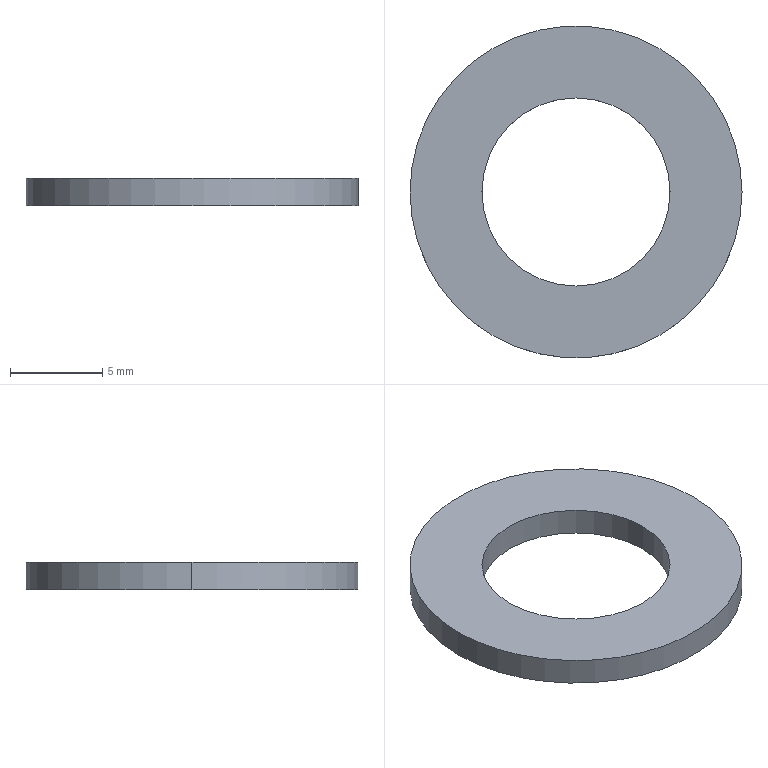Part | SolidWorks | features Extrusion 1 | 1 solid | 6 faces | box 18 x 18 x 1.5 mm | volume 259.134 mm3 | cylinder 4 | plane 2 | commonest cylinder face diameters 10.2 x2 18 x2
STEP:
#1=CARTESIAN_POINT('',(-5.1,0.,-0.75));
#2=VERTEX_POINT('',#1);
#3=CARTESIAN_POINT('',(5.1,0.,-0.75));
#4=VERTEX_POINT('',#3);
#5=CARTESIAN_POINT('',(0.,0.,-0.75));
#6=DIRECTION('',(0.,0.,1.));
#7=DIRECTION('',(1.,0.,0.));
#8=AXIS2_PLACEMENT_3D('',#5,#6,#7);
#9=CIRCLE('',#8,5.1);
#10=EDGE_CURVE('',#2,#4,#9,.T.);
#11=ORIENTED_EDGE('',*,*,#10,.F.);
#12=CARTESIAN_POINT('',(-5.1,0.,0.75));
#13=VERTEX_POINT('',#12);
#14=CARTESIAN_POINT('',(-5.1,0.,-0.75));
#15=DIRECTION('',(0.,0.,1.));
#16=VECTOR('',#15,1000.);
#17=LINE('',#14,#16);
#18=EDGE_CURVE('',#2,#13,#17,.T.);
#19=ORIENTED_EDGE('',*,*,#18,.T.);
#20=CARTESIAN_POINT('',(5.1,0.,0.75));
#21=VERTEX_POINT('',#20);
#22=CARTESIAN_POINT('',(0.,0.,0.75));
#23=DIRECTION('',(0.,0.,1.));
#24=DIRECTION('',(1.,0.,0.));
#25=AXIS2_PLACEMENT_3D('',#22,#23,#24);
#26=CIRCLE('',#25,5.1);
#27=EDGE_CURVE('',#13,#21,#26,.T.);
#28=ORIENTED_EDGE('',*,*,#27,.T.);
#29=CARTESIAN_POINT('',(5.1,0.,-0.75));
#30=DIRECTION('',(0.,0.,1.));
#31=VECTOR('',#30,1000.);
#32=LINE('',#29,#31);
#33=EDGE_CURVE('',#4,#21,#32,.T.);
#34=ORIENTED_EDGE('',*,*,#33,.F.);
#35=EDGE_LOOP('',(#11,#19,#28,#34));
#36=FACE_OUTER_BOUND('',#35,.T.);
#37=CARTESIAN_POINT('',(0.,0.,-0.75));
#38=DIRECTION('',(0.,0.,1.));
#39=DIRECTION('',(1.,0.,0.));
#40=AXIS2_PLACEMENT_3D('',#37,#38,#39);
#41=CYLINDRICAL_SURFACE('',#40,5.1);
#42=ADVANCED_FACE('',(#36),#41,.F.);
#43=CARTESIAN_POINT('',(9.,0.,-0.75));
#44=VERTEX_POINT('',#43);
#45=CARTESIAN_POINT('',(-9.,0.,-0.75));
#46=VERTEX_POINT('',#45);
#47=CARTESIAN_POINT('',(0.,0.,-0.75));
#48=DIRECTION('',(0.,0.,1.));
#49=DIRECTION('',(1.,0.,0.));
#50=AXIS2_PLACEMENT_3D('',#47,#48,#49);
#51=CIRCLE('',#50,9.);
#52=EDGE_CURVE('',#44,#46,#51,.T.);
#53=ORIENTED_EDGE('',*,*,#52,.T.);
#54=CARTESIAN_POINT('',(-9.,0.,0.75));
#55=VERTEX_POINT('',#54);
#56=CARTESIAN_POINT('',(-9.,0.,-0.75));
#57=DIRECTION('',(0.,0.,1.));
#58=VECTOR('',#57,1000.);
#59=LINE('',#56,#58);
#60=EDGE_CURVE('',#46,#55,#59,.T.);
#61=ORIENTED_EDGE('',*,*,#60,.T.);
#62=CARTESIAN_POINT('',(9.,0.,0.75));
#63=VERTEX_POINT('',#62);
#64=CARTESIAN_POINT('',(0.,0.,0.75));
#65=DIRECTION('',(0.,0.,1.));
#66=DIRECTION('',(1.,0.,0.));
#67=AXIS2_PLACEMENT_3D('',#64,#65,#66);
#68=CIRCLE('',#67,9.);
#69=EDGE_CURVE('',#63,#55,#68,.T.);
#70=ORIENTED_EDGE('',*,*,#69,.F.);
#71=CARTESIAN_POINT('',(9.,0.,-0.75));
#72=DIRECTION('',(0.,0.,1.));
#73=VECTOR('',#72,1000.);
#74=LINE('',#71,#73);
#75=EDGE_CURVE('',#44,#63,#74,.T.);
#76=ORIENTED_EDGE('',*,*,#75,.F.);
#77=EDGE_LOOP('',(#53,#61,#70,#76));
#78=FACE_OUTER_BOUND('',#77,.T.);
#79=CARTESIAN_POINT('',(0.,0.,-0.75));
#80=DIRECTION('',(0.,0.,1.));
#81=DIRECTION('',(1.,0.,0.));
#82=AXIS2_PLACEMENT_3D('',#79,#80,#81);
#83=CYLINDRICAL_SURFACE('',#82,9.);
#84=ADVANCED_FACE('',(#78),#83,.T.);
#85=ORIENTED_EDGE('',*,*,#60,.F.);
#86=CARTESIAN_POINT('',(0.,0.,-0.75));
#87=DIRECTION('',(0.,0.,1.));
#88=DIRECTION('',(1.,0.,0.));
#89=AXIS2_PLACEMENT_3D('',#86,#87,#88);
#90=CIRCLE('',#89,9.);
#91=EDGE_CURVE('',#46,#44,#90,.T.);
#92=ORIENTED_EDGE('',*,*,#91,.T.);
#93=ORIENTED_EDGE('',*,*,#75,.T.);
#94=CARTESIAN_POINT('',(0.,0.,0.75));
#95=DIRECTION('',(0.,0.,1.));
#96=DIRECTION('',(1.,0.,0.));
#97=AXIS2_PLACEMENT_3D('',#94,#95,#96);
#98=CIRCLE('',#97,9.);
#99=EDGE_CURVE('',#55,#63,#98,.T.);
#100=ORIENTED_EDGE('',*,*,#99,.F.);
#101=EDGE_LOOP('',(#85,#92,#93,#100));
#102=FACE_OUTER_BOUND('',#101,.T.);
#103=CARTESIAN_POINT('',(0.,0.,-0.75));
#104=DIRECTION('',(0.,0.,1.));
#105=DIRECTION('',(1.,0.,0.));
#106=AXIS2_PLACEMENT_3D('',#103,#104,#105);
#107=CYLINDRICAL_SURFACE('',#106,9.);
#108=ADVANCED_FACE('',(#102),#107,.T.);
#109=CARTESIAN_POINT('',(0.,0.,-0.75));
#110=DIRECTION('',(0.,0.,1.));
#111=DIRECTION('',(1.,0.,0.));
#112=AXIS2_PLACEMENT_3D('',#109,#110,#111);
#113=CIRCLE('',#112,5.1);
#114=EDGE_CURVE('',#4,#2,#113,.T.);
#115=ORIENTED_EDGE('',*,*,#114,.T.);
#116=ORIENTED_EDGE('',*,*,#10,.T.);
#117=EDGE_LOOP('',(#115,#116));
#118=FACE_BOUND('',#117,.T.);
#119=ORIENTED_EDGE('',*,*,#52,.F.);
#120=ORIENTED_EDGE('',*,*,#91,.F.);
#121=EDGE_LOOP('',(#119,#120));
#122=FACE_OUTER_BOUND('',#121,.T.);
#123=CARTESIAN_POINT('',(0.,0.,-0.75));
#124=DIRECTION('',(0.,0.,1.));
#125=DIRECTION('',(1.,0.,0.));
#126=AXIS2_PLACEMENT_3D('',#123,#124,#125);
#127=PLANE('',#126);
#128=ADVANCED_FACE('',(#118,#122),#127,.F.);
#129=CARTESIAN_POINT('',(0.,0.,0.75));
#130=DIRECTION('',(0.,0.,1.));
#131=DIRECTION('',(1.,0.,0.));
#132=AXIS2_PLACEMENT_3D('',#129,#130,#131);
#133=CIRCLE('',#132,5.1);
#134=EDGE_CURVE('',#21,#13,#133,.T.);
#135=ORIENTED_EDGE('',*,*,#134,.F.);
#136=ORIENTED_EDGE('',*,*,#27,.F.);
#137=EDGE_LOOP('',(#135,#136));
#138=FACE_BOUND('',#137,.T.);
#139=ORIENTED_EDGE('',*,*,#69,.T.);
#140=ORIENTED_EDGE('',*,*,#99,.T.);
#141=EDGE_LOOP('',(#139,#140));
#142=FACE_OUTER_BOUND('',#141,.T.);
#143=CARTESIAN_POINT('',(0.,0.,0.75));
#144=DIRECTION('',(0.,0.,1.));
#145=DIRECTION('',(1.,0.,0.));
#146=AXIS2_PLACEMENT_3D('',#143,#144,#145);
#147=PLANE('',#146);
#148=ADVANCED_FACE('',(#138,#142),#147,.T.);
#149=ORIENTED_EDGE('',*,*,#18,.F.);
#150=ORIENTED_EDGE('',*,*,#114,.F.);
#151=ORIENTED_EDGE('',*,*,#33,.T.);
#152=ORIENTED_EDGE('',*,*,#134,.T.);
#153=EDGE_LOOP('',(#149,#150,#151,#152));
#154=FACE_OUTER_BOUND('',#153,.T.);
#155=CARTESIAN_POINT('',(0.,0.,-0.75));
#156=DIRECTION('',(0.,0.,1.));
#157=DIRECTION('',(1.,0.,0.));
#158=AXIS2_PLACEMENT_3D('',#155,#156,#157);
#159=CYLINDRICAL_SURFACE('',#158,5.1);
#160=ADVANCED_FACE('',(#154),#159,.F.);
#161=CLOSED_SHELL('',(#42,#84,#108,#128,#148,#160));
#162=MANIFOLD_SOLID_BREP('',#161);
#163=CARTESIAN_POINT('',(0.,0.,0.));
#164=DIRECTION('',(0.,0.,1.));
#165=DIRECTION('',(1.,0.,0.));
#166=AXIS2_PLACEMENT_3D('',#163,#164,#165);
#167=(LENGTH_UNIT()NAMED_UNIT(*)SI_UNIT(.MILLI.,.METRE.));
#168=UNCERTAINTY_MEASURE_WITH_UNIT(LENGTH_MEASURE(0.00001),#167,'','');
#169=(NAMED_UNIT(*)PLANE_ANGLE_UNIT()SI_UNIT($,.RADIAN.));
#170=(NAMED_UNIT(*)SI_UNIT($,.STERADIAN.)SOLID_ANGLE_UNIT());
#171=(GEOMETRIC_REPRESENTATION_CONTEXT(3)GLOBAL_UNCERTAINTY_ASSIGNED_CONTEXT((#168))GLOBAL_UNIT_ASSIGNED_CONTEXT((#167,#169,#170))REPRESENTATION_CONTEXT('',''));
#172=ADVANCED_BREP_SHAPE_REPRESENTATION('',(#162,#166),#171);